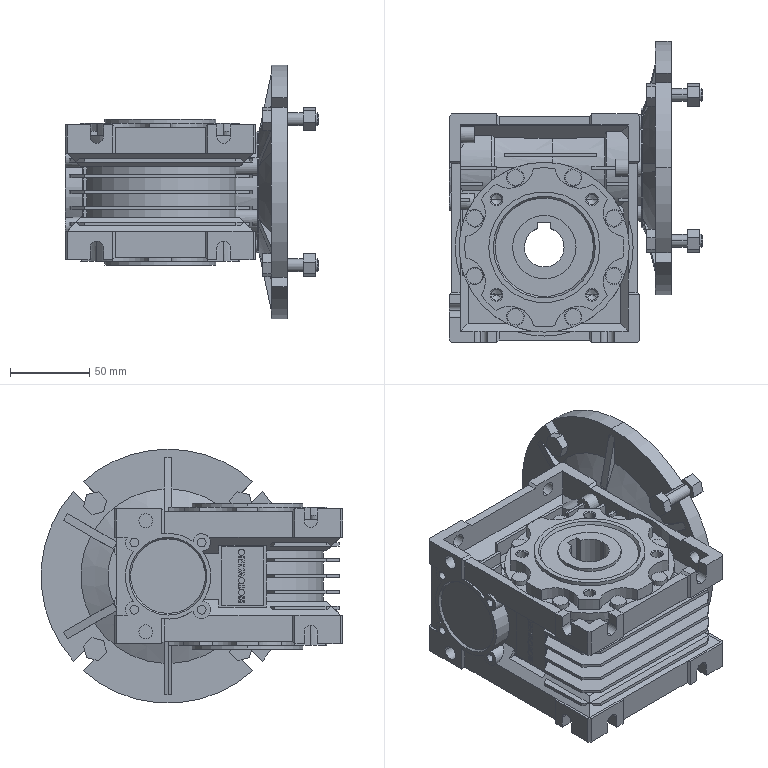Part | SolidWorks | features BaseBody 9 | 9 solids | 1092 faces | box 160 x 190.03 x 160.06 mm | volume 1157137 mm3 | plane 648 | cylinder 306 | cone 109 | spline 29 | commonest cylinder face diameters 11 x47 10 x28 61 x19 100 x18 6.647 x16 8 x16